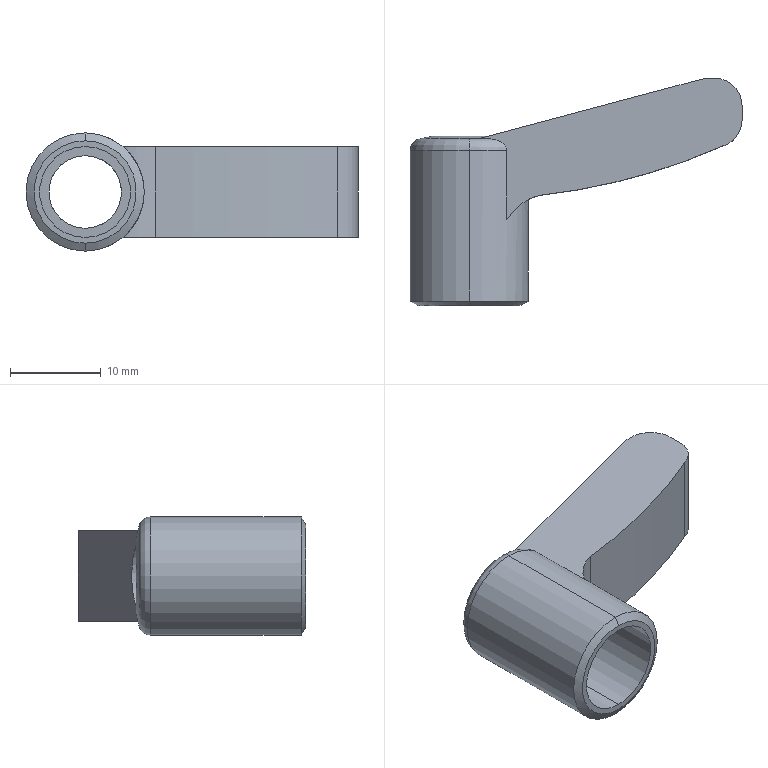Part | SolidWorks | features RefAxis 3, 3DProfileFeature 1, ICE 1, RevCut 1, Revolution 1 | 1 solid | 24 faces | box 36.5 x 25 x 13 mm | volume 3149 mm3 | cylinder 10 | plane 7 | torus 3 | cone 2 | sphere 2 | commonest cylinder face diameters 6 x2 8 x2 10 x2 13 x2 12 x1 135.84 x1
STEP:
#1=CARTESIAN_POINT('',(0.,17.156,-4.));
#2=VERTEX_POINT('',#1);
#3=CARTESIAN_POINT('',(0.,17.156,4.));
#4=VERTEX_POINT('',#3);
#5=CARTESIAN_POINT('',(0.,17.156,0.));
#6=DIRECTION('',(0.,1.,0.));
#7=DIRECTION('',(0.,0.,1.));
#8=AXIS2_PLACEMENT_3D('',#5,#6,#7);
#9=CIRCLE('',#8,4.);
#10=EDGE_CURVE('',#2,#4,#9,.T.);
#11=ORIENTED_EDGE('',*,*,#10,.F.);
#12=CARTESIAN_POINT('',(0.,22.63,-4.));
#13=VERTEX_POINT('',#12);
#14=CARTESIAN_POINT('',(0.,-2.644,-4.));
#15=DIRECTION('',(0.,1.,0.));
#16=VECTOR('',#15,1000.);
#17=LINE('',#14,#16);
#18=EDGE_CURVE('',#2,#13,#17,.T.);
#19=ORIENTED_EDGE('',*,*,#18,.T.);
#20=CARTESIAN_POINT('',(-4.,22.63,0.));
#21=VERTEX_POINT('',#20);
#22=CARTESIAN_POINT('',(0.,22.63,0.));
#23=DIRECTION('',(0.,1.,0.));
#24=DIRECTION('',(0.,0.,-1.));
#25=AXIS2_PLACEMENT_3D('',#22,#23,#24);
#26=CIRCLE('',#25,4.);
#27=EDGE_CURVE('',#13,#21,#26,.T.);
#28=ORIENTED_EDGE('',*,*,#27,.T.);
#29=CARTESIAN_POINT('',(0.,22.63,4.));
#30=VERTEX_POINT('',#29);
#31=CARTESIAN_POINT('',(0.,22.63,0.));
#32=DIRECTION('',(0.,1.,0.));
#33=DIRECTION('',(0.,0.,-1.));
#34=AXIS2_PLACEMENT_3D('',#31,#32,#33);
#35=CIRCLE('',#34,4.);
#36=EDGE_CURVE('',#21,#30,#35,.T.);
#37=ORIENTED_EDGE('',*,*,#36,.T.);
#38=CARTESIAN_POINT('',(0.,-2.644,4.));
#39=DIRECTION('',(0.,1.,0.));
#40=VECTOR('',#39,1000.);
#41=LINE('',#38,#40);
#42=EDGE_CURVE('',#4,#30,#41,.T.);
#43=ORIENTED_EDGE('',*,*,#42,.F.);
#44=EDGE_LOOP('',(#11,#19,#28,#37,#43));
#45=FACE_OUTER_BOUND('',#44,.T.);
#46=CARTESIAN_POINT('',(0.,-2.644,0.));
#47=DIRECTION('',(0.,1.,0.));
#48=DIRECTION('',(0.,0.,1.));
#49=AXIS2_PLACEMENT_3D('',#46,#47,#48);
#50=CYLINDRICAL_SURFACE('',#49,4.);
#51=ADVANCED_FACE('',(#45),#50,.F.);
#52=CARTESIAN_POINT('',(0.,4.,5.));
#53=VERTEX_POINT('',#52);
#54=CARTESIAN_POINT('',(0.,4.,-5.));
#55=VERTEX_POINT('',#54);
#56=CARTESIAN_POINT('',(0.,4.,0.));
#57=DIRECTION('',(0.,-1.,0.));
#58=DIRECTION('',(0.,0.,1.));
#59=AXIS2_PLACEMENT_3D('',#56,#57,#58);
#60=CIRCLE('',#59,5.);
#61=EDGE_CURVE('',#53,#55,#60,.T.);
#62=ORIENTED_EDGE('',*,*,#61,.T.);
#63=CARTESIAN_POINT('',(0.,17.156,-5.));
#64=VERTEX_POINT('',#63);
#65=CARTESIAN_POINT('',(0.,-2.644,-5.));
#66=DIRECTION('',(0.,1.,0.));
#67=VECTOR('',#66,1000.);
#68=LINE('',#65,#67);
#69=EDGE_CURVE('',#55,#64,#68,.T.);
#70=ORIENTED_EDGE('',*,*,#69,.T.);
#71=CARTESIAN_POINT('',(0.,17.156,5.));
#72=VERTEX_POINT('',#71);
#73=CARTESIAN_POINT('',(0.,17.156,0.));
#74=DIRECTION('',(0.,1.,0.));
#75=DIRECTION('',(0.,0.,1.));
#76=AXIS2_PLACEMENT_3D('',#73,#74,#75);
#77=CIRCLE('',#76,5.);
#78=EDGE_CURVE('',#64,#72,#77,.T.);
#79=ORIENTED_EDGE('',*,*,#78,.T.);
#80=CARTESIAN_POINT('',(0.,-2.644,5.));
#81=DIRECTION('',(0.,1.,0.));
#82=VECTOR('',#81,1000.);
#83=LINE('',#80,#82);
#84=EDGE_CURVE('',#53,#72,#83,.T.);
#85=ORIENTED_EDGE('',*,*,#84,.F.);
#86=EDGE_LOOP('',(#62,#70,#79,#85));
#87=FACE_OUTER_BOUND('',#86,.T.);
#88=CARTESIAN_POINT('',(0.,-2.644,0.));
#89=DIRECTION('',(0.,1.,0.));
#90=DIRECTION('',(0.,0.,1.));
#91=AXIS2_PLACEMENT_3D('',#88,#89,#90);
#92=CYLINDRICAL_SURFACE('',#91,5.);
#93=ADVANCED_FACE('',(#87),#92,.F.);
#94=CARTESIAN_POINT('',(0.,4.,5.634));
#95=VERTEX_POINT('',#94);
#96=CARTESIAN_POINT('',(0.,4.,-5.634));
#97=VERTEX_POINT('',#96);
#98=CARTESIAN_POINT('',(0.,4.,0.));
#99=DIRECTION('',(0.,1.,0.));
#100=DIRECTION('',(0.,0.,1.));
#101=AXIS2_PLACEMENT_3D('',#98,#99,#100);
#102=CIRCLE('',#101,5.634);
#103=EDGE_CURVE('',#95,#97,#102,.T.);
#104=ORIENTED_EDGE('',*,*,#103,.T.);
#105=CARTESIAN_POINT('',(0.,4.5,-6.5));
#106=VERTEX_POINT('',#105);
#107=CARTESIAN_POINT('',(0.,4.,-5.634));
#108=DIRECTION('',(0.,0.5,-0.866));
#109=VECTOR('',#108,1000.);
#110=LINE('',#107,#109);
#111=EDGE_CURVE('',#97,#106,#110,.T.);
#112=ORIENTED_EDGE('',*,*,#111,.T.);
#113=CARTESIAN_POINT('',(0.,4.5,6.5));
#114=VERTEX_POINT('',#113);
#115=CARTESIAN_POINT('',(0.,4.5,0.));
#116=DIRECTION('',(0.,1.,0.));
#117=DIRECTION('',(0.,0.,1.));
#118=AXIS2_PLACEMENT_3D('',#115,#116,#117);
#119=CIRCLE('',#118,6.5);
#120=EDGE_CURVE('',#114,#106,#119,.T.);
#121=ORIENTED_EDGE('',*,*,#120,.F.);
#122=CARTESIAN_POINT('',(0.,4.,5.634));
#123=DIRECTION('',(0.,0.5,0.866));
#124=VECTOR('',#123,1000.);
#125=LINE('',#122,#124);
#126=EDGE_CURVE('',#95,#114,#125,.T.);
#127=ORIENTED_EDGE('',*,*,#126,.F.);
#128=EDGE_LOOP('',(#104,#112,#121,#127));
#129=FACE_OUTER_BOUND('',#128,.T.);
#130=CARTESIAN_POINT('',(0.,4.,0.));
#131=DIRECTION('',(0.,1.,0.));
#132=DIRECTION('',(0.,0.,1.));
#133=AXIS2_PLACEMENT_3D('',#130,#131,#132);
#134=CONICAL_SURFACE('',#133,5.634,1.047);
#135=ADVANCED_FACE('',(#129),#134,.T.);
#136=ORIENTED_EDGE('',*,*,#120,.T.);
#137=CARTESIAN_POINT('',(0.,21.057,-6.5));
#138=VERTEX_POINT('',#137);
#139=CARTESIAN_POINT('',(0.,4.,-6.5));
#140=DIRECTION('',(0.,1.,0.));
#141=VECTOR('',#140,1000.);
#142=LINE('',#139,#141);
#143=EDGE_CURVE('',#106,#138,#142,.T.);
#144=ORIENTED_EDGE('',*,*,#143,.T.);
#145=CARTESIAN_POINT('',(4.153,21.057,-5.));
#146=VERTEX_POINT('',#145);
#147=CARTESIAN_POINT('',(0.,21.057,0.));
#148=DIRECTION('',(0.,1.,0.));
#149=DIRECTION('',(0.,0.,1.));
#150=AXIS2_PLACEMENT_3D('',#147,#148,#149);
#151=CIRCLE('',#150,6.5);
#152=EDGE_CURVE('',#146,#138,#151,.T.);
#153=ORIENTED_EDGE('',*,*,#152,.F.);
#154=CARTESIAN_POINT('',(4.153,13.493,-5.));
#155=VERTEX_POINT('',#154);
#156=CARTESIAN_POINT('',(4.153,4.,-5.));
#157=DIRECTION('',(0.,-1.,0.));
#158=VECTOR('',#157,1000.);
#159=LINE('',#156,#158);
#160=EDGE_CURVE('',#146,#155,#159,.T.);
#161=ORIENTED_EDGE('',*,*,#160,.T.);
#162=CARTESIAN_POINT('',(4.153,13.493,5.));
#163=VERTEX_POINT('',#162);
#164=CARTESIAN_POINT('',(4.153,13.493,5.));
#165=CARTESIAN_POINT('',(4.41,13.906,4.787));
#166=CARTESIAN_POINT('',(4.695,14.253,4.518));
#167=CARTESIAN_POINT('',(5.266,14.832,3.836));
#168=CARTESIAN_POINT('',(5.538,15.049,3.441));
#169=CARTESIAN_POINT('',(6.002,15.379,2.546));
#170=CARTESIAN_POINT('',(6.186,15.487,2.065));
#171=CARTESIAN_POINT('',(6.437,15.628,1.045));
#172=CARTESIAN_POINT('',(6.5,15.659,0.5239));
#173=CARTESIAN_POINT('',(6.5,15.659,-0.2665));
#174=CARTESIAN_POINT('',(6.483,15.651,-0.5323));
#175=CARTESIAN_POINT('',(6.42,15.617,-1.052));
#176=CARTESIAN_POINT('',(6.372,15.592,-1.308));
#177=CARTESIAN_POINT('',(6.248,15.522,-1.812));
#178=CARTESIAN_POINT('',(6.17,15.477,-2.061));
#179=CARTESIAN_POINT('',(5.987,15.363,-2.544));
#180=CARTESIAN_POINT('',(5.883,15.295,-2.775));
#181=CARTESIAN_POINT('',(5.655,15.132,-3.215));
#182=CARTESIAN_POINT('',(5.53,15.037,-3.425));
#183=CARTESIAN_POINT('',(5.263,14.814,-3.822));
#184=CARTESIAN_POINT('',(5.122,14.685,-4.008));
#185=CARTESIAN_POINT('',(4.84,14.4,-4.344));
#186=CARTESIAN_POINT('',(4.698,14.242,-4.497));
#187=CARTESIAN_POINT('',(4.418,13.891,-4.771));
#188=CARTESIAN_POINT('',(4.28,13.697,-4.894));
#189=CARTESIAN_POINT('',(4.153,13.493,-5.));
#190=B_SPLINE_CURVE_WITH_KNOTS('',3,(#164,#165,#166,#167,#168,#169,#170,#171,#172,#173,#174,#175,#176,#177,#178,#179,#180,#181,#182,#183,#184,#185,#186,#187,#188,#189),.UNSPECIFIED.,.F.,.F.,(4,2,2,2,2,2,2,2,2,2,2,2,4),(0.003403,0.004974,0.006546,0.008117,0.009688,0.01047,0.01126,0.01205,0.01283,0.01362,0.0144,0.01519,0.01597),.UNSPECIFIED.);
#191=EDGE_CURVE('',#163,#155,#190,.T.);
#192=ORIENTED_EDGE('',*,*,#191,.F.);
#193=CARTESIAN_POINT('',(4.153,21.057,5.));
#194=VERTEX_POINT('',#193);
#195=CARTESIAN_POINT('',(4.153,4.,5.));
#196=DIRECTION('',(0.,-1.,0.));
#197=VECTOR('',#196,1000.);
#198=LINE('',#195,#197);
#199=EDGE_CURVE('',#194,#163,#198,.T.);
#200=ORIENTED_EDGE('',*,*,#199,.F.);
#201=CARTESIAN_POINT('',(0.,21.057,6.5));
#202=VERTEX_POINT('',#201);
#203=CARTESIAN_POINT('',(0.,21.057,0.));
#204=DIRECTION('',(0.,1.,0.));
#205=DIRECTION('',(0.,0.,1.));
#206=AXIS2_PLACEMENT_3D('',#203,#204,#205);
#207=CIRCLE('',#206,6.5);
#208=EDGE_CURVE('',#202,#194,#207,.T.);
#209=ORIENTED_EDGE('',*,*,#208,.F.);
#210=CARTESIAN_POINT('',(0.,4.,6.5));
#211=DIRECTION('',(0.,1.,0.));
#212=VECTOR('',#211,1000.);
#213=LINE('',#210,#212);
#214=EDGE_CURVE('',#114,#202,#213,.T.);
#215=ORIENTED_EDGE('',*,*,#214,.F.);
#216=EDGE_LOOP('',(#136,#144,#153,#161,#192,#200,#209,#215));
#217=FACE_OUTER_BOUND('',#216,.T.);
#218=CARTESIAN_POINT('',(0.,4.,0.));
#219=DIRECTION('',(0.,1.,0.));
#220=DIRECTION('',(0.,0.,1.));
#221=AXIS2_PLACEMENT_3D('',#218,#219,#220);
#222=CYLINDRICAL_SURFACE('',#221,6.5);
#223=ADVANCED_FACE('',(#217),#222,.T.);
#224=ORIENTED_EDGE('',*,*,#152,.T.);
#225=CARTESIAN_POINT('',(0.,22.322,-5.503));
#226=VERTEX_POINT('',#225);
#227=CARTESIAN_POINT('',(0.,21.057,-5.2));
#228=DIRECTION('',(1.,0.,0.));
#229=DIRECTION('',(0.,0.,-1.));
#230=AXIS2_PLACEMENT_3D('',#227,#228,#229);
#231=CIRCLE('',#230,1.3);
#232=EDGE_CURVE('',#138,#226,#231,.T.);
#233=ORIENTED_EDGE('',*,*,#232,.T.);
#234=CARTESIAN_POINT('',(2.298,22.322,-5.));
#235=VERTEX_POINT('',#234);
#236=CARTESIAN_POINT('',(0.,22.322,0.));
#237=DIRECTION('',(0.,1.,0.));
#238=DIRECTION('',(0.,0.,1.));
#239=AXIS2_PLACEMENT_3D('',#236,#237,#238);
#240=CIRCLE('',#239,5.503);
#241=EDGE_CURVE('',#235,#226,#240,.T.);
#242=ORIENTED_EDGE('',*,*,#241,.F.);
#243=CARTESIAN_POINT('',(2.298,22.322,-5.));
#244=CARTESIAN_POINT('',(2.5,22.301,-5.));
#245=CARTESIAN_POINT('',(2.701,22.27,-5.));
#246=CARTESIAN_POINT('',(3.098,22.171,-5.));
#247=CARTESIAN_POINT('',(3.293,22.103,-5.));
#248=CARTESIAN_POINT('',(3.564,21.958,-5.));
#249=CARTESIAN_POINT('',(3.65,21.903,-5.));
#250=CARTESIAN_POINT('',(3.809,21.777,-5.));
#251=CARTESIAN_POINT('',(3.884,21.705,-5.));
#252=CARTESIAN_POINT('',(4.073,21.463,-5.));
#253=CARTESIAN_POINT('',(4.153,21.263,-5.));
#254=CARTESIAN_POINT('',(4.153,21.057,-5.));
#255=B_SPLINE_CURVE_WITH_KNOTS('',3,(#243,#244,#245,#246,#247,#248,#249,#250,#251,#252,#253,#254),.UNSPECIFIED.,.F.,.F.,(4,2,2,2,2,4),(0.0006992,0.001308,0.001917,0.002221,0.002525,0.003134),.UNSPECIFIED.);
#256=EDGE_CURVE('',#235,#146,#255,.T.);
#257=ORIENTED_EDGE('',*,*,#256,.T.);
#258=EDGE_LOOP('',(#224,#233,#242,#257));
#259=FACE_OUTER_BOUND('',#258,.T.);
#260=CARTESIAN_POINT('',(0.,21.057,0.));
#261=DIRECTION('',(0.,1.,0.));
#262=DIRECTION('',(0.,0.,1.));
#263=AXIS2_PLACEMENT_3D('',#260,#261,#262);
#264=TOROIDAL_SURFACE('',#263,5.2,1.3);
#265=ADVANCED_FACE('',(#259),#264,.T.);
#266=ORIENTED_EDGE('',*,*,#232,.F.);
#267=CARTESIAN_POINT('',(0.,21.057,0.));
#268=DIRECTION('',(0.,1.,0.));
#269=DIRECTION('',(0.,0.,1.));
#270=AXIS2_PLACEMENT_3D('',#267,#268,#269);
#271=CIRCLE('',#270,6.5);
#272=EDGE_CURVE('',#138,#202,#271,.T.);
#273=ORIENTED_EDGE('',*,*,#272,.T.);
#274=CARTESIAN_POINT('',(0.,22.322,5.503));
#275=VERTEX_POINT('',#274);
#276=CARTESIAN_POINT('',(0.,21.057,5.2));
#277=DIRECTION('',(-1.,0.,0.));
#278=DIRECTION('',(0.,0.,1.));
#279=AXIS2_PLACEMENT_3D('',#276,#277,#278);
#280=CIRCLE('',#279,1.3);
#281=EDGE_CURVE('',#202,#275,#280,.T.);
#282=ORIENTED_EDGE('',*,*,#281,.T.);
#283=CARTESIAN_POINT('',(-5.503,22.322,0.));
#284=VERTEX_POINT('',#283);
#285=CARTESIAN_POINT('',(0.,22.322,0.));
#286=DIRECTION('',(0.,1.,0.));
#287=DIRECTION('',(0.,0.,1.));
#288=AXIS2_PLACEMENT_3D('',#285,#286,#287);
#289=CIRCLE('',#288,5.503);
#290=EDGE_CURVE('',#284,#275,#289,.T.);
#291=ORIENTED_EDGE('',*,*,#290,.F.);
#292=CARTESIAN_POINT('',(0.,22.322,0.));
#293=DIRECTION('',(0.,1.,0.));
#294=DIRECTION('',(0.,0.,1.));
#295=AXIS2_PLACEMENT_3D('',#292,#293,#294);
#296=CIRCLE('',#295,5.503);
#297=EDGE_CURVE('',#226,#284,#296,.T.);
#298=ORIENTED_EDGE('',*,*,#297,.F.);
#299=EDGE_LOOP('',(#266,#273,#282,#291,#298));
#300=FACE_OUTER_BOUND('',#299,.T.);
#301=CARTESIAN_POINT('',(0.,21.057,0.));
#302=DIRECTION('',(0.,1.,0.));
#303=DIRECTION('',(0.,0.,1.));
#304=AXIS2_PLACEMENT_3D('',#301,#302,#303);
#305=TOROIDAL_SURFACE('',#304,5.2,1.3);
#306=ADVANCED_FACE('',(#300),#305,.T.);
#307=ORIENTED_EDGE('',*,*,#241,.T.);
#308=ORIENTED_EDGE('',*,*,#297,.T.);
#309=CARTESIAN_POINT('',(0.,-0.6437,0.));
#310=DIRECTION('',(0.,0.,-1.));
#311=DIRECTION('',(-1.,0.,0.));
#312=AXIS2_PLACEMENT_3D('',#309,#310,#311);
#313=CIRCLE('',#312,23.615);
#314=EDGE_CURVE('',#284,#21,#313,.T.);
#315=ORIENTED_EDGE('',*,*,#314,.T.);
#316=ORIENTED_EDGE('',*,*,#27,.F.);
#317=CARTESIAN_POINT('',(2.161,22.63,-3.366));
#318=VERTEX_POINT('',#317);
#319=CARTESIAN_POINT('',(0.,22.63,0.));
#320=DIRECTION('',(0.,1.,0.));
#321=DIRECTION('',(0.,0.,-1.));
#322=AXIS2_PLACEMENT_3D('',#319,#320,#321);
#323=CIRCLE('',#322,4.);
#324=EDGE_CURVE('',#318,#13,#323,.T.);
#325=ORIENTED_EDGE('',*,*,#324,.F.);
#326=CARTESIAN_POINT('',(1.3,22.4,-5.));
#327=VERTEX_POINT('',#326);
#328=CARTESIAN_POINT('',(-5.674,20.531,0.));
#329=DIRECTION('',(0.2588,-0.9659,0.));
#330=DIRECTION('',(0.9659,0.2588,0.));
#331=AXIS2_PLACEMENT_3D('',#328,#329,#330);
#332=CIRCLE('',#331,8.782);
#333=EDGE_CURVE('',#327,#318,#332,.T.);
#334=ORIENTED_EDGE('',*,*,#333,.F.);
#335=CARTESIAN_POINT('',(0.,-0.6437,-5.));
#336=DIRECTION('',(0.,0.,-1.));
#337=DIRECTION('',(-1.,0.,0.));
#338=AXIS2_PLACEMENT_3D('',#335,#336,#337);
#339=CIRCLE('',#338,23.08);
#340=EDGE_CURVE('',#327,#235,#339,.T.);
#341=ORIENTED_EDGE('',*,*,#340,.T.);
#342=EDGE_LOOP('',(#307,#308,#315,#316,#325,#334,#341));
#343=FACE_OUTER_BOUND('',#342,.T.);
#344=CARTESIAN_POINT('',(0.,-0.6437,0.));
#345=DIRECTION('',(0.,0.,-1.));
#346=DIRECTION('',(1.,0.,0.));
#347=AXIS2_PLACEMENT_3D('',#344,#345,#346);
#348=SPHERICAL_SURFACE('',#347,23.615);
#349=ADVANCED_FACE('',(#343),#348,.T.);
#350=ORIENTED_EDGE('',*,*,#314,.F.);
#351=ORIENTED_EDGE('',*,*,#290,.T.);
#352=CARTESIAN_POINT('',(2.298,22.322,5.));
#353=VERTEX_POINT('',#352);
#354=CARTESIAN_POINT('',(0.,22.322,0.));
#355=DIRECTION('',(0.,1.,0.));
#356=DIRECTION('',(0.,0.,1.));
#357=AXIS2_PLACEMENT_3D('',#354,#355,#356);
#358=CIRCLE('',#357,5.503);
#359=EDGE_CURVE('',#275,#353,#358,.T.);
#360=ORIENTED_EDGE('',*,*,#359,.T.);
#361=CARTESIAN_POINT('',(1.3,22.4,5.));
#362=VERTEX_POINT('',#361);
#363=CARTESIAN_POINT('',(0.,-0.6437,5.));
#364=DIRECTION('',(0.,0.,-1.));
#365=DIRECTION('',(-1.,0.,0.));
#366=AXIS2_PLACEMENT_3D('',#363,#364,#365);
#367=CIRCLE('',#366,23.08);
#368=EDGE_CURVE('',#362,#353,#367,.T.);
#369=ORIENTED_EDGE('',*,*,#368,.F.);
#370=CARTESIAN_POINT('',(2.161,22.63,3.366));
#371=VERTEX_POINT('',#370);
#372=CARTESIAN_POINT('',(-5.674,20.531,0.));
#373=DIRECTION('',(0.2588,-0.9659,0.));
#374=DIRECTION('',(0.9659,0.2588,0.));
#375=AXIS2_PLACEMENT_3D('',#372,#373,#374);
#376=CIRCLE('',#375,8.782);
#377=EDGE_CURVE('',#371,#362,#376,.T.);
#378=ORIENTED_EDGE('',*,*,#377,.F.);
#379=CARTESIAN_POINT('',(0.,22.63,0.));
#380=DIRECTION('',(0.,1.,0.));
#381=DIRECTION('',(0.,0.,-1.));
#382=AXIS2_PLACEMENT_3D('',#379,#380,#381);
#383=CIRCLE('',#382,4.);
#384=EDGE_CURVE('',#30,#371,#383,.T.);
#385=ORIENTED_EDGE('',*,*,#384,.F.);
#386=ORIENTED_EDGE('',*,*,#36,.F.);
#387=EDGE_LOOP('',(#350,#351,#360,#369,#378,#385,#386));
#388=FACE_OUTER_BOUND('',#387,.T.);
#389=CARTESIAN_POINT('',(0.,-0.6437,0.));
#390=DIRECTION('',(0.,0.,-1.));
#391=DIRECTION('',(1.,0.,0.));
#392=AXIS2_PLACEMENT_3D('',#389,#390,#391);
#393=SPHERICAL_SURFACE('',#392,23.615);
#394=ADVANCED_FACE('',(#388),#393,.T.);
#395=ORIENTED_EDGE('',*,*,#103,.F.);
#396=CARTESIAN_POINT('',(0.,4.,0.));
#397=DIRECTION('',(0.,1.,0.));
#398=DIRECTION('',(0.,0.,1.));
#399=AXIS2_PLACEMENT_3D('',#396,#397,#398);
#400=CIRCLE('',#399,5.634);
#401=EDGE_CURVE('',#97,#95,#400,.T.);
#402=ORIENTED_EDGE('',*,*,#401,.F.);
#403=EDGE_LOOP('',(#395,#402));
#404=FACE_OUTER_BOUND('',#403,.T.);
#405=ORIENTED_EDGE('',*,*,#61,.F.);
#406=CARTESIAN_POINT('',(0.,4.,0.));
#407=DIRECTION('',(0.,-1.,0.));
#408=DIRECTION('',(0.,0.,1.));
#409=AXIS2_PLACEMENT_3D('',#406,#407,#408);
#410=CIRCLE('',#409,5.);
#411=EDGE_CURVE('',#55,#53,#410,.T.);
#412=ORIENTED_EDGE('',*,*,#411,.F.);
#413=EDGE_LOOP('',(#405,#412));
#414=FACE_BOUND('',#413,.T.);
#415=CARTESIAN_POINT('',(5.634,4.,0.));
#416=DIRECTION('',(0.,1.,0.));
#417=DIRECTION('',(0.,0.,1.));
#418=AXIS2_PLACEMENT_3D('',#415,#416,#417);
#419=PLANE('',#418);
#420=ADVANCED_FACE('',(#404,#414),#419,.F.);
#421=CARTESIAN_POINT('',(2.161,22.63,3.366));
#422=CARTESIAN_POINT('',(4.884,23.36,1.618));
#423=CARTESIAN_POINT('',(4.884,23.36,-1.618));
#424=CARTESIAN_POINT('',(2.161,22.63,-3.366));
#425=(BOUNDED_CURVE()B_SPLINE_CURVE(3,(#421,#422,#423,#424),.UNSPECIFIED.,.F.,.T.)B_SPLINE_CURVE_WITH_KNOTS((4,4),(5.283,7.283),.UNSPECIFIED.)CURVE()GEOMETRIC_REPRESENTATION_ITEM()RATIONAL_B_SPLINE_CURVE((1.,0.6936,0.6936,1.))REPRESENTATION_ITEM(''));
#426=EDGE_CURVE('',#371,#318,#425,.T.);
#427=ORIENTED_EDGE('',*,*,#426,.F.);
#428=ORIENTED_EDGE('',*,*,#377,.T.);
#429=CARTESIAN_POINT('',(25.933,29.,5.));
#430=VERTEX_POINT('',#429);
#431=CARTESIAN_POINT('',(25.933,29.,5.));
#432=DIRECTION('',(-0.9659,-0.2588,0.));
#433=VECTOR('',#432,1000.);
#434=LINE('',#431,#433);
#435=EDGE_CURVE('',#430,#362,#434,.T.);
#436=ORIENTED_EDGE('',*,*,#435,.F.);
#437=CARTESIAN_POINT('',(25.933,29.,-5.));
#438=VERTEX_POINT('',#437);
#439=CARTESIAN_POINT('',(25.933,29.,5.));
#440=DIRECTION('',(0.,0.,-1.));
#441=VECTOR('',#440,1000.);
#442=LINE('',#439,#441);
#443=EDGE_CURVE('',#430,#438,#442,.T.);
#444=ORIENTED_EDGE('',*,*,#443,.T.);
#445=CARTESIAN_POINT('',(25.933,29.,-5.));
#446=DIRECTION('',(-0.9659,-0.2588,0.));
#447=VECTOR('',#446,1000.);
#448=LINE('',#445,#447);
#449=EDGE_CURVE('',#438,#327,#448,.T.);
#450=ORIENTED_EDGE('',*,*,#449,.T.);
#451=ORIENTED_EDGE('',*,*,#333,.T.);
#452=EDGE_LOOP('',(#427,#428,#436,#444,#450,#451));
#453=FACE_OUTER_BOUND('',#452,.T.);
#454=CARTESIAN_POINT('',(25.933,29.,5.));
#455=DIRECTION('',(0.2588,-0.9659,0.));
#456=DIRECTION('',(0.9659,0.2588,0.));
#457=AXIS2_PLACEMENT_3D('',#454,#455,#456);
#458=PLANE('',#457);
#459=ADVANCED_FACE('',(#453),#458,.F.);
#460=ORIENTED_EDGE('',*,*,#281,.F.);
#461=ORIENTED_EDGE('',*,*,#208,.T.);
#462=CARTESIAN_POINT('',(2.298,22.322,5.));
#463=CARTESIAN_POINT('',(2.5,22.301,5.));
#464=CARTESIAN_POINT('',(2.701,22.27,5.));
#465=CARTESIAN_POINT('',(3.098,22.171,5.));
#466=CARTESIAN_POINT('',(3.293,22.103,5.));
#467=CARTESIAN_POINT('',(3.564,21.958,5.));
#468=CARTESIAN_POINT('',(3.65,21.903,5.));
#469=CARTESIAN_POINT('',(3.809,21.777,5.));
#470=CARTESIAN_POINT('',(3.884,21.705,5.));
#471=CARTESIAN_POINT('',(4.073,21.463,5.));
#472=CARTESIAN_POINT('',(4.153,21.263,5.));
#473=CARTESIAN_POINT('',(4.153,21.057,5.));
#474=B_SPLINE_CURVE_WITH_KNOTS('',3,(#462,#463,#464,#465,#466,#467,#468,#469,#470,#471,#472,#473),.UNSPECIFIED.,.F.,.F.,(4,2,2,2,2,4),(0.0006992,0.001308,0.001917,0.002221,0.002525,0.003134),.UNSPECIFIED.);
#475=EDGE_CURVE('',#353,#194,#474,.T.);
#476=ORIENTED_EDGE('',*,*,#475,.F.);
#477=ORIENTED_EDGE('',*,*,#359,.F.);
#478=EDGE_LOOP('',(#460,#461,#476,#477));
#479=FACE_OUTER_BOUND('',#478,.T.);
#480=CARTESIAN_POINT('',(0.,21.057,0.));
#481=DIRECTION('',(0.,1.,0.));
#482=DIRECTION('',(0.,0.,1.));
#483=AXIS2_PLACEMENT_3D('',#480,#481,#482);
#484=TOROIDAL_SURFACE('',#483,5.2,1.3);
#485=ADVANCED_FACE('',(#479),#484,.T.);
#486=ORIENTED_EDGE('',*,*,#143,.F.);
#487=CARTESIAN_POINT('',(0.,4.5,0.));
#488=DIRECTION('',(0.,1.,0.));
#489=DIRECTION('',(0.,0.,1.));
#490=AXIS2_PLACEMENT_3D('',#487,#488,#489);
#491=CIRCLE('',#490,6.5);
#492=EDGE_CURVE('',#106,#114,#491,.T.);
#493=ORIENTED_EDGE('',*,*,#492,.T.);
#494=ORIENTED_EDGE('',*,*,#214,.T.);
#495=ORIENTED_EDGE('',*,*,#272,.F.);
#496=EDGE_LOOP('',(#486,#493,#494,#495));
#497=FACE_OUTER_BOUND('',#496,.T.);
#498=CARTESIAN_POINT('',(0.,4.,0.));
#499=DIRECTION('',(0.,1.,0.));
#500=DIRECTION('',(0.,0.,1.));
#501=AXIS2_PLACEMENT_3D('',#498,#499,#500);
#502=CYLINDRICAL_SURFACE('',#501,6.5);
#503=ADVANCED_FACE('',(#497),#502,.T.);
#504=ORIENTED_EDGE('',*,*,#111,.F.);
#505=ORIENTED_EDGE('',*,*,#401,.T.);
#506=ORIENTED_EDGE('',*,*,#126,.T.);
#507=ORIENTED_EDGE('',*,*,#492,.F.);
#508=EDGE_LOOP('',(#504,#505,#506,#507));
#509=FACE_OUTER_BOUND('',#508,.T.);
#510=CARTESIAN_POINT('',(0.,4.,0.));
#511=DIRECTION('',(0.,1.,0.));
#512=DIRECTION('',(0.,0.,1.));
#513=AXIS2_PLACEMENT_3D('',#510,#511,#512);
#514=CONICAL_SURFACE('',#513,5.634,1.047);
#515=ADVANCED_FACE('',(#509),#514,.T.);
#516=CARTESIAN_POINT('',(7.697,16.122,5.));
#517=VERTEX_POINT('',#516);
#518=CARTESIAN_POINT('',(9.25,10.327,5.));
#519=DIRECTION('',(0.,0.,-1.));
#520=DIRECTION('',(-1.,0.,0.));
#521=AXIS2_PLACEMENT_3D('',#518,#519,#520);
#522=CIRCLE('',#521,6.);
#523=EDGE_CURVE('',#163,#517,#522,.T.);
#524=ORIENTED_EDGE('',*,*,#523,.F.);
#525=ORIENTED_EDGE('',*,*,#191,.T.);
#526=CARTESIAN_POINT('',(7.697,16.122,-5.));
#527=VERTEX_POINT('',#526);
#528=CARTESIAN_POINT('',(9.25,10.327,-5.));
#529=DIRECTION('',(0.,0.,-1.));
#530=DIRECTION('',(-1.,0.,0.));
#531=AXIS2_PLACEMENT_3D('',#528,#529,#530);
#532=CIRCLE('',#531,6.);
#533=EDGE_CURVE('',#155,#527,#532,.T.);
#534=ORIENTED_EDGE('',*,*,#533,.T.);
#535=CARTESIAN_POINT('',(7.697,16.122,5.));
#536=DIRECTION('',(0.,0.,-1.));
#537=VECTOR('',#536,1000.);
#538=LINE('',#535,#537);
#539=EDGE_CURVE('',#517,#527,#538,.T.);
#540=ORIENTED_EDGE('',*,*,#539,.F.);
#541=EDGE_LOOP('',(#524,#525,#534,#540));
#542=FACE_OUTER_BOUND('',#541,.T.);
#543=CARTESIAN_POINT('',(9.25,10.327,5.));
#544=DIRECTION('',(0.,0.,-1.));
#545=DIRECTION('',(-1.,0.,0.));
#546=AXIS2_PLACEMENT_3D('',#543,#544,#545);
#547=CYLINDRICAL_SURFACE('',#546,6.);
#548=ADVANCED_FACE('',(#542),#547,.F.);
#549=ORIENTED_EDGE('',*,*,#435,.T.);
#550=ORIENTED_EDGE('',*,*,#368,.T.);
#551=ORIENTED_EDGE('',*,*,#475,.T.);
#552=ORIENTED_EDGE('',*,*,#199,.T.);
#553=ORIENTED_EDGE('',*,*,#523,.T.);
#554=CARTESIAN_POINT('',(27.776,21.502,5.));
#555=VERTEX_POINT('',#554);
#556=CARTESIAN_POINT('',(0.3648,83.645,5.));
#557=DIRECTION('',(0.,0.,1.));
#558=DIRECTION('',(1.,0.,0.));
#559=AXIS2_PLACEMENT_3D('',#556,#557,#558);
#560=CIRCLE('',#559,67.92);
#561=EDGE_CURVE('',#517,#555,#560,.T.);
#562=ORIENTED_EDGE('',*,*,#561,.T.);
#563=CARTESIAN_POINT('',(30.,24.4,5.));
#564=VERTEX_POINT('',#563);
#565=CARTESIAN_POINT('',(27.,24.4,5.));
#566=DIRECTION('',(0.,0.,1.));
#567=DIRECTION('',(1.,0.,0.));
#568=AXIS2_PLACEMENT_3D('',#565,#566,#567);
#569=CIRCLE('',#568,3.);
#570=EDGE_CURVE('',#555,#564,#569,.T.);
#571=ORIENTED_EDGE('',*,*,#570,.T.);
#572=CARTESIAN_POINT('',(30.,26.,5.));
#573=VERTEX_POINT('',#572);
#574=CARTESIAN_POINT('',(30.,24.4,5.));
#575=DIRECTION('',(0.,1.,0.));
#576=VECTOR('',#575,1000.);
#577=LINE('',#574,#576);
#578=EDGE_CURVE('',#564,#573,#577,.T.);
#579=ORIENTED_EDGE('',*,*,#578,.T.);
#580=CARTESIAN_POINT('',(27.,29.,5.));
#581=VERTEX_POINT('',#580);
#582=CARTESIAN_POINT('',(27.,26.,5.));
#583=DIRECTION('',(0.,0.,1.));
#584=DIRECTION('',(1.,0.,0.));
#585=AXIS2_PLACEMENT_3D('',#582,#583,#584);
#586=CIRCLE('',#585,3.);
#587=EDGE_CURVE('',#573,#581,#586,.T.);
#588=ORIENTED_EDGE('',*,*,#587,.T.);
#589=CARTESIAN_POINT('',(27.,29.,5.));
#590=DIRECTION('',(-1.,0.,0.));
#591=VECTOR('',#590,1000.);
#592=LINE('',#589,#591);
#593=EDGE_CURVE('',#581,#430,#592,.T.);
#594=ORIENTED_EDGE('',*,*,#593,.T.);
#595=EDGE_LOOP('',(#549,#550,#551,#552,#553,#562,#571,#579,#588,#594));
#596=FACE_OUTER_BOUND('',#595,.T.);
#597=CARTESIAN_POINT('',(9.25,10.327,5.));
#598=DIRECTION('',(0.,0.,-1.));
#599=DIRECTION('',(-1.,0.,0.));
#600=AXIS2_PLACEMENT_3D('',#597,#598,#599);
#601=PLANE('',#600);
#602=ADVANCED_FACE('',(#596),#601,.F.);
#603=ORIENTED_EDGE('',*,*,#340,.F.);
#604=ORIENTED_EDGE('',*,*,#449,.F.);
#605=CARTESIAN_POINT('',(27.,29.,-5.));
#606=VERTEX_POINT('',#605);
#607=CARTESIAN_POINT('',(27.,29.,-5.));
#608=DIRECTION('',(-1.,0.,0.));
#609=VECTOR('',#608,1000.);
#610=LINE('',#607,#609);
#611=EDGE_CURVE('',#606,#438,#610,.T.);
#612=ORIENTED_EDGE('',*,*,#611,.F.);
#613=CARTESIAN_POINT('',(30.,26.,-5.));
#614=VERTEX_POINT('',#613);
#615=CARTESIAN_POINT('',(27.,26.,-5.));
#616=DIRECTION('',(0.,0.,1.));
#617=DIRECTION('',(1.,0.,0.));
#618=AXIS2_PLACEMENT_3D('',#615,#616,#617);
#619=CIRCLE('',#618,3.);
#620=EDGE_CURVE('',#614,#606,#619,.T.);
#621=ORIENTED_EDGE('',*,*,#620,.F.);
#622=CARTESIAN_POINT('',(30.,24.4,-5.));
#623=VERTEX_POINT('',#622);
#624=CARTESIAN_POINT('',(30.,24.4,-5.));
#625=DIRECTION('',(0.,1.,0.));
#626=VECTOR('',#625,1000.);
#627=LINE('',#624,#626);
#628=EDGE_CURVE('',#623,#614,#627,.T.);
#629=ORIENTED_EDGE('',*,*,#628,.F.);
#630=CARTESIAN_POINT('',(27.776,21.502,-5.));
#631=VERTEX_POINT('',#630);
#632=CARTESIAN_POINT('',(27.,24.4,-5.));
#633=DIRECTION('',(0.,0.,1.));
#634=DIRECTION('',(1.,0.,0.));
#635=AXIS2_PLACEMENT_3D('',#632,#633,#634);
#636=CIRCLE('',#635,3.);
#637=EDGE_CURVE('',#631,#623,#636,.T.);
#638=ORIENTED_EDGE('',*,*,#637,.F.);
#639=CARTESIAN_POINT('',(0.3648,83.645,-5.));
#640=DIRECTION('',(0.,0.,1.));
#641=DIRECTION('',(1.,0.,0.));
#642=AXIS2_PLACEMENT_3D('',#639,#640,#641);
#643=CIRCLE('',#642,67.92);
#644=EDGE_CURVE('',#527,#631,#643,.T.);
#645=ORIENTED_EDGE('',*,*,#644,.F.);
#646=ORIENTED_EDGE('',*,*,#533,.F.);
#647=ORIENTED_EDGE('',*,*,#160,.F.);
#648=ORIENTED_EDGE('',*,*,#256,.F.);
#649=EDGE_LOOP('',(#603,#604,#612,#621,#629,#638,#645,#646,#647,#648));
#650=FACE_OUTER_BOUND('',#649,.T.);
#651=CARTESIAN_POINT('',(9.25,10.327,-5.));
#652=DIRECTION('',(0.,0.,-1.));
#653=DIRECTION('',(-1.,0.,0.));
#654=AXIS2_PLACEMENT_3D('',#651,#652,#653);
#655=PLANE('',#654);
#656=ADVANCED_FACE('',(#650),#655,.T.);
#657=ORIENTED_EDGE('',*,*,#539,.T.);
#658=ORIENTED_EDGE('',*,*,#644,.T.);
#659=CARTESIAN_POINT('',(27.776,21.502,5.));
#660=DIRECTION('',(0.,0.,-1.));
#661=VECTOR('',#660,1000.);
#662=LINE('',#659,#661);
#663=EDGE_CURVE('',#555,#631,#662,.T.);
#664=ORIENTED_EDGE('',*,*,#663,.F.);
#665=ORIENTED_EDGE('',*,*,#561,.F.);
#666=EDGE_LOOP('',(#657,#658,#664,#665));
#667=FACE_OUTER_BOUND('',#666,.T.);
#668=CARTESIAN_POINT('',(0.3648,83.645,5.));
#669=DIRECTION('',(0.,0.,-1.));
#670=DIRECTION('',(-1.,0.,0.));
#671=AXIS2_PLACEMENT_3D('',#668,#669,#670);
#672=CYLINDRICAL_SURFACE('',#671,67.92);
#673=ADVANCED_FACE('',(#667),#672,.T.);
#674=ORIENTED_EDGE('',*,*,#663,.T.);
#675=ORIENTED_EDGE('',*,*,#637,.T.);
#676=CARTESIAN_POINT('',(30.,24.4,5.));
#677=DIRECTION('',(0.,0.,-1.));
#678=VECTOR('',#677,1000.);
#679=LINE('',#676,#678);
#680=EDGE_CURVE('',#564,#623,#679,.T.);
#681=ORIENTED_EDGE('',*,*,#680,.F.);
#682=ORIENTED_EDGE('',*,*,#570,.F.);
#683=EDGE_LOOP('',(#674,#675,#681,#682));
#684=FACE_OUTER_BOUND('',#683,.T.);
#685=CARTESIAN_POINT('',(27.,24.4,5.));
#686=DIRECTION('',(0.,0.,-1.));
#687=DIRECTION('',(-1.,0.,0.));
#688=AXIS2_PLACEMENT_3D('',#685,#686,#687);
#689=CYLINDRICAL_SURFACE('',#688,3.);
#690=ADVANCED_FACE('',(#684),#689,.T.);
#691=ORIENTED_EDGE('',*,*,#680,.T.);
#692=ORIENTED_EDGE('',*,*,#628,.T.);
#693=CARTESIAN_POINT('',(30.,26.,5.));
#694=DIRECTION('',(0.,0.,-1.));
#695=VECTOR('',#694,1000.);
#696=LINE('',#693,#695);
#697=EDGE_CURVE('',#573,#614,#696,.T.);
#698=ORIENTED_EDGE('',*,*,#697,.F.);
#699=ORIENTED_EDGE('',*,*,#578,.F.);
#700=EDGE_LOOP('',(#691,#692,#698,#699));
#701=FACE_OUTER_BOUND('',#700,.T.);
#702=CARTESIAN_POINT('',(30.,24.4,5.));
#703=DIRECTION('',(-1.,0.,0.));
#704=DIRECTION('',(0.,0.,1.));
#705=AXIS2_PLACEMENT_3D('',#702,#703,#704);
#706=PLANE('',#705);
#707=ADVANCED_FACE('',(#701),#706,.F.);
#708=ORIENTED_EDGE('',*,*,#697,.T.);
#709=ORIENTED_EDGE('',*,*,#620,.T.);
#710=CARTESIAN_POINT('',(27.,29.,5.));
#711=DIRECTION('',(0.,0.,-1.));
#712=VECTOR('',#711,1000.);
#713=LINE('',#710,#712);
#714=EDGE_CURVE('',#581,#606,#713,.T.);
#715=ORIENTED_EDGE('',*,*,#714,.F.);
#716=ORIENTED_EDGE('',*,*,#587,.F.);
#717=EDGE_LOOP('',(#708,#709,#715,#716));
#718=FACE_OUTER_BOUND('',#717,.T.);
#719=CARTESIAN_POINT('',(27.,26.,5.));
#720=DIRECTION('',(0.,0.,-1.));
#721=DIRECTION('',(-1.,0.,0.));
#722=AXIS2_PLACEMENT_3D('',#719,#720,#721);
#723=CYLINDRICAL_SURFACE('',#722,3.);
#724=ADVANCED_FACE('',(#718),#723,.T.);
#725=ORIENTED_EDGE('',*,*,#714,.T.);
#726=ORIENTED_EDGE('',*,*,#611,.T.);
#727=ORIENTED_EDGE('',*,*,#443,.F.);
#728=ORIENTED_EDGE('',*,*,#593,.F.);
#729=EDGE_LOOP('',(#725,#726,#727,#728));
#730=FACE_OUTER_BOUND('',#729,.T.);
#731=CARTESIAN_POINT('',(27.,29.,5.));
#732=DIRECTION('',(0.,-1.,0.));
#733=DIRECTION('',(0.,0.,-1.));
#734=AXIS2_PLACEMENT_3D('',#731,#732,#733);
#735=PLANE('',#734);
#736=ADVANCED_FACE('',(#730),#735,.F.);
#737=ORIENTED_EDGE('',*,*,#69,.F.);
#738=ORIENTED_EDGE('',*,*,#411,.T.);
#739=ORIENTED_EDGE('',*,*,#84,.T.);
#740=CARTESIAN_POINT('',(0.,17.156,0.));
#741=DIRECTION('',(0.,1.,0.));
#742=DIRECTION('',(0.,0.,1.));
#743=AXIS2_PLACEMENT_3D('',#740,#741,#742);
#744=CIRCLE('',#743,5.);
#745=EDGE_CURVE('',#72,#64,#744,.T.);
#746=ORIENTED_EDGE('',*,*,#745,.T.);
#747=EDGE_LOOP('',(#737,#738,#739,#746));
#748=FACE_OUTER_BOUND('',#747,.T.);
#749=CARTESIAN_POINT('',(0.,-2.644,0.));
#750=DIRECTION('',(0.,1.,0.));
#751=DIRECTION('',(0.,0.,1.));
#752=AXIS2_PLACEMENT_3D('',#749,#750,#751);
#753=CYLINDRICAL_SURFACE('',#752,5.);
#754=ADVANCED_FACE('',(#748),#753,.F.);
#755=ORIENTED_EDGE('',*,*,#18,.F.);
#756=CARTESIAN_POINT('',(0.,17.156,0.));
#757=DIRECTION('',(0.,1.,0.));
#758=DIRECTION('',(0.,0.,1.));
#759=AXIS2_PLACEMENT_3D('',#756,#757,#758);
#760=CIRCLE('',#759,4.);
#761=EDGE_CURVE('',#4,#2,#760,.T.);
#762=ORIENTED_EDGE('',*,*,#761,.F.);
#763=ORIENTED_EDGE('',*,*,#42,.T.);
#764=ORIENTED_EDGE('',*,*,#384,.T.);
#765=ORIENTED_EDGE('',*,*,#426,.T.);
#766=ORIENTED_EDGE('',*,*,#324,.T.);
#767=EDGE_LOOP('',(#755,#762,#763,#764,#765,#766));
#768=FACE_OUTER_BOUND('',#767,.T.);
#769=CARTESIAN_POINT('',(0.,-2.644,0.));
#770=DIRECTION('',(0.,1.,0.));
#771=DIRECTION('',(0.,0.,1.));
#772=AXIS2_PLACEMENT_3D('',#769,#770,#771);
#773=CYLINDRICAL_SURFACE('',#772,4.);
#774=ADVANCED_FACE('',(#768),#773,.F.);
#775=ORIENTED_EDGE('',*,*,#761,.T.);
#776=ORIENTED_EDGE('',*,*,#10,.T.);
#777=EDGE_LOOP('',(#775,#776));
#778=FACE_BOUND('',#777,.T.);
#779=ORIENTED_EDGE('',*,*,#745,.F.);
#780=ORIENTED_EDGE('',*,*,#78,.F.);
#781=EDGE_LOOP('',(#779,#780));
#782=FACE_OUTER_BOUND('',#781,.T.);
#783=CARTESIAN_POINT('',(4.,17.156,0.));
#784=DIRECTION('',(0.,-1.,0.));
#785=DIRECTION('',(0.,0.,-1.));
#786=AXIS2_PLACEMENT_3D('',#783,#784,#785);
#787=PLANE('',#786);
#788=ADVANCED_FACE('',(#778,#782),#787,.T.);
#789=CLOSED_SHELL('',(#51,#93,#135,#223,#265,#306,#349,#394,#420,#459,#485,#503,#515,#548,#602,#656,#673,#690,#707,#724,#736,#754,#774,#788));
#790=MANIFOLD_SOLID_BREP('',#789);
#791=CARTESIAN_POINT('',(0.,0.,0.));
#792=DIRECTION('',(0.,0.,1.));
#793=DIRECTION('',(1.,0.,0.));
#794=AXIS2_PLACEMENT_3D('',#791,#792,#793);
#795=(LENGTH_UNIT()NAMED_UNIT(*)SI_UNIT(.MILLI.,.METRE.));
#796=UNCERTAINTY_MEASURE_WITH_UNIT(LENGTH_MEASURE(0.00001),#795,'','');
#797=(NAMED_UNIT(*)PLANE_ANGLE_UNIT()SI_UNIT($,.RADIAN.));
#798=(NAMED_UNIT(*)SI_UNIT($,.STERADIAN.)SOLID_ANGLE_UNIT());
#799=(GEOMETRIC_REPRESENTATION_CONTEXT(3)GLOBAL_UNCERTAINTY_ASSIGNED_CONTEXT((#796))GLOBAL_UNIT_ASSIGNED_CONTEXT((#795,#797,#798))REPRESENTATION_CONTEXT('',''));
#800=ADVANCED_BREP_SHAPE_REPRESENTATION('',(#790,#794),#799);